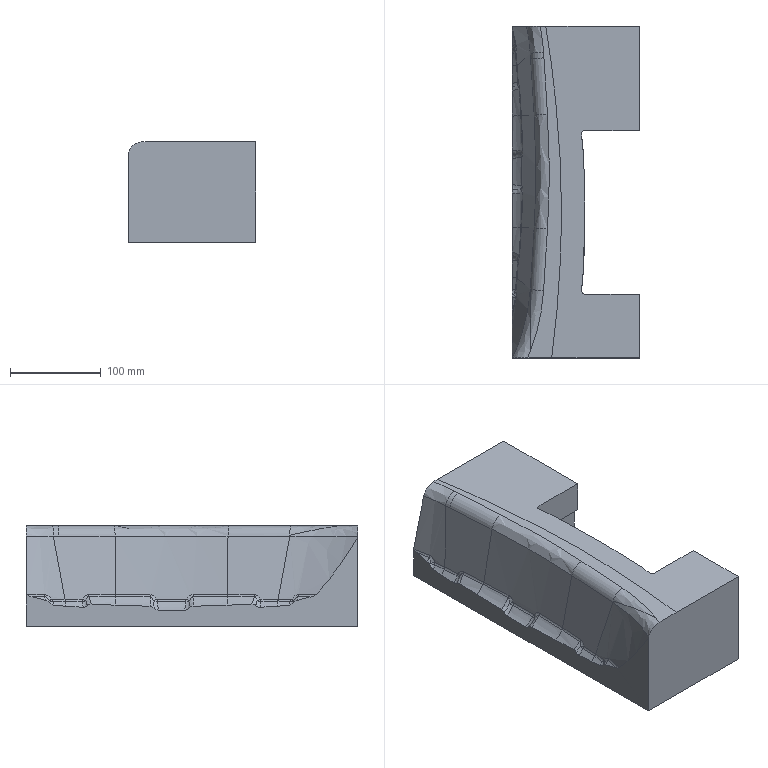Part | NX | features solid 2 | 1 solid | 73 faces | box 140.004 x 365 x 111 mm | volume 4062417 mm3 | spline 66 | plane 7